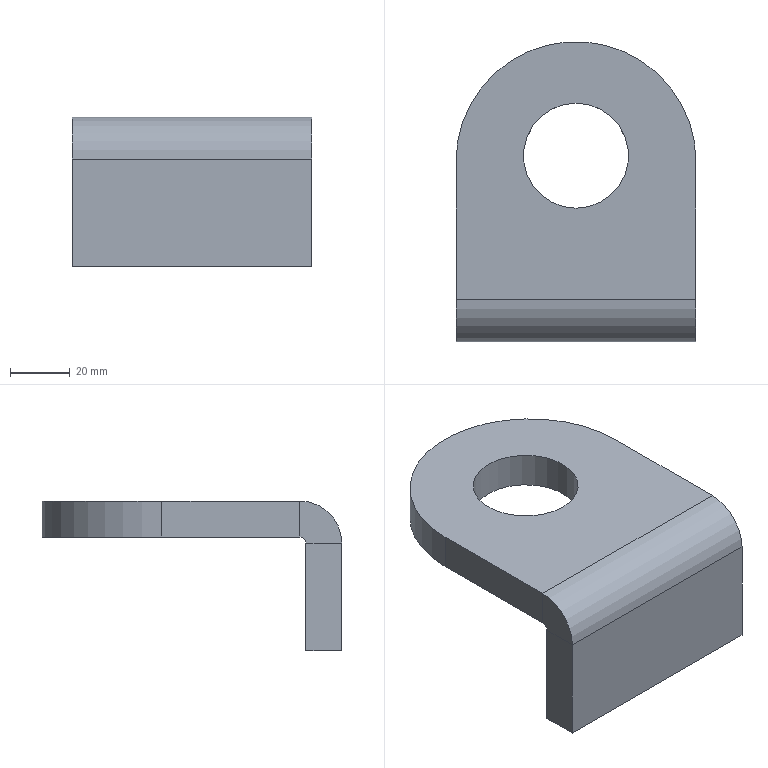Part | STEP file | PN_0019 lifting lug _Default<As Machined> | 1 solid | 15 faces | box 80 x 100 x 50 mm | volume 109398 mm3 | plane 11 | cylinder 4 | commonest cylinder face diameters 4 x1 28 x1 35 x1 80 x1
STEP:
#1=CARTESIAN_POINT('',(0.,0.,0.));
#2=DIRECTION('',(0.,0.,1.));
#3=DIRECTION('',(1.,0.,0.));
#4=AXIS2_PLACEMENT_3D('',#1,#2,#3);
#5=CARTESIAN_POINT('',(-40.,48.,25.));
#6=VERTEX_POINT('',#5);
#7=CARTESIAN_POINT('',(-40.,48.,13.));
#8=VERTEX_POINT('',#7);
#9=CARTESIAN_POINT('',(-40.,48.,25.));
#10=DIRECTION('',(0.,0.,-1.));
#11=VECTOR('',#10,1.);
#12=LINE('',#9,#11);
#13=CARTESIAN_POINT('',(0.,48.,25.));
#14=DIRECTION('',(0.,0.,-1.));
#15=DIRECTION('',(0.,1.,0.));
#16=AXIS2_PLACEMENT_3D('',#13,#14,#15);
#17=CYLINDRICAL_SURFACE('',#16,40.);
#18=CARTESIAN_POINT('',(4.712,0.));
#19=DIRECTION('',(0.,1.));
#20=VECTOR('',#19,1.);
#21=LINE('',#18,#20);
#22=(GEOMETRIC_REPRESENTATION_CONTEXT(2)PARAMETRIC_REPRESENTATION_CONTEXT()REPRESENTATION_CONTEXT('',''));
#23=DEFINITIONAL_REPRESENTATION('',(#21),#22);
#24=PCURVE('',#17,#23);
#25=CARTESIAN_POINT('',(-40.,88.,25.));
#26=DIRECTION('',(-1.,0.,0.));
#27=DIRECTION('',(0.,-1.,0.));
#28=AXIS2_PLACEMENT_3D('',#25,#26,#27);
#29=PLANE('',#28);
#30=CARTESIAN_POINT('',(40.,0.));
#31=DIRECTION('',(0.,-1.));
#32=VECTOR('',#31,1.);
#33=LINE('',#30,#32);
#34=(GEOMETRIC_REPRESENTATION_CONTEXT(2)PARAMETRIC_REPRESENTATION_CONTEXT()REPRESENTATION_CONTEXT('',''));
#35=DEFINITIONAL_REPRESENTATION('',(#33),#34);
#36=PCURVE('',#29,#35);
#37=SURFACE_CURVE('',#12,(#24,#36),.PCURVE_S1.);
#38=EDGE_CURVE('',#6,#8,#37,.T.);
#39=ORIENTED_EDGE('',*,*,#38,.F.);
#40=CARTESIAN_POINT('',(40.,48.,25.));
#41=VERTEX_POINT('',#40);
#42=CARTESIAN_POINT('',(0.,48.,25.));
#43=DIRECTION('',(0.,0.,1.));
#44=DIRECTION('',(0.,-1.,0.));
#45=AXIS2_PLACEMENT_3D('',#42,#43,#44);
#46=CIRCLE('',#45,40.);
#47=CARTESIAN_POINT('',(9.425,0.));
#48=DIRECTION('',(-1.,0.));
#49=VECTOR('',#48,1.);
#50=LINE('',#47,#49);
#51=(GEOMETRIC_REPRESENTATION_CONTEXT(2)PARAMETRIC_REPRESENTATION_CONTEXT()REPRESENTATION_CONTEXT('',''));
#52=DEFINITIONAL_REPRESENTATION('',(#50),#51);
#53=PCURVE('',#17,#52);
#54=CARTESIAN_POINT('',(0.,0.,25.));
#55=DIRECTION('',(0.,0.,1.));
#56=DIRECTION('',(0.,-1.,0.));
#57=AXIS2_PLACEMENT_3D('',#54,#55,#56);
#58=PLANE('',#57);
#59=CARTESIAN_POINT('',(-48.,0.));
#60=DIRECTION('',(1.,0.));
#61=AXIS2_PLACEMENT_2D('',#59,#60);
#62=CIRCLE('',#61,40.);
#63=(GEOMETRIC_REPRESENTATION_CONTEXT(2)PARAMETRIC_REPRESENTATION_CONTEXT()REPRESENTATION_CONTEXT('',''));
#64=DEFINITIONAL_REPRESENTATION('',(#62),#63);
#65=PCURVE('',#58,#64);
#66=SURFACE_CURVE('',#46,(#53,#65),.PCURVE_S1.);
#67=EDGE_CURVE('',#41,#6,#66,.T.);
#68=ORIENTED_EDGE('',*,*,#67,.F.);
#69=CARTESIAN_POINT('',(40.,48.,13.));
#70=VERTEX_POINT('',#69);
#71=CARTESIAN_POINT('',(40.,48.,25.));
#72=DIRECTION('',(0.,0.,1.));
#73=VECTOR('',#72,1.);
#74=LINE('',#71,#73);
#75=CARTESIAN_POINT('',(7.854,0.));
#76=DIRECTION('',(0.,-1.));
#77=VECTOR('',#76,1.);
#78=LINE('',#75,#77);
#79=(GEOMETRIC_REPRESENTATION_CONTEXT(2)PARAMETRIC_REPRESENTATION_CONTEXT()REPRESENTATION_CONTEXT('',''));
#80=DEFINITIONAL_REPRESENTATION('',(#78),#79);
#81=PCURVE('',#17,#80);
#82=CARTESIAN_POINT('',(40.,0.,25.));
#83=DIRECTION('',(1.,0.,0.));
#84=DIRECTION('',(0.,1.,0.));
#85=AXIS2_PLACEMENT_3D('',#82,#83,#84);
#86=PLANE('',#85);
#87=CARTESIAN_POINT('',(48.,0.));
#88=DIRECTION('',(0.,1.));
#89=VECTOR('',#88,1.);
#90=LINE('',#87,#89);
#91=(GEOMETRIC_REPRESENTATION_CONTEXT(2)PARAMETRIC_REPRESENTATION_CONTEXT()REPRESENTATION_CONTEXT('',''));
#92=DEFINITIONAL_REPRESENTATION('',(#90),#91);
#93=PCURVE('',#86,#92);
#94=SURFACE_CURVE('',#74,(#81,#93),.PCURVE_S1.);
#95=EDGE_CURVE('',#70,#41,#94,.T.);
#96=ORIENTED_EDGE('',*,*,#95,.F.);
#97=CARTESIAN_POINT('',(0.,48.,13.));
#98=DIRECTION('',(0.,0.,-1.));
#99=DIRECTION('',(0.,-1.,0.));
#100=AXIS2_PLACEMENT_3D('',#97,#98,#99);
#101=CIRCLE('',#100,40.);
#102=CARTESIAN_POINT('',(3.142,12.));
#103=DIRECTION('',(1.,0.));
#104=VECTOR('',#103,1.);
#105=LINE('',#102,#104);
#106=(GEOMETRIC_REPRESENTATION_CONTEXT(2)PARAMETRIC_REPRESENTATION_CONTEXT()REPRESENTATION_CONTEXT('',''));
#107=DEFINITIONAL_REPRESENTATION('',(#105),#106);
#108=PCURVE('',#17,#107);
#109=CARTESIAN_POINT('',(0.,0.,13.));
#110=DIRECTION('',(0.,0.,1.));
#111=DIRECTION('',(0.,-1.,0.));
#112=AXIS2_PLACEMENT_3D('',#109,#110,#111);
#113=PLANE('',#112);
#114=CARTESIAN_POINT('',(-8.,0.));
#115=CARTESIAN_POINT('',(-8.,-69.282));
#116=CARTESIAN_POINT('',(-68.,-34.641));
#117=CARTESIAN_POINT('',(-128.,0.));
#118=CARTESIAN_POINT('',(-68.,34.641));
#119=CARTESIAN_POINT('',(-8.,69.282));
#120=CARTESIAN_POINT('',(-8.,0.));
#121=(BOUNDED_CURVE()B_SPLINE_CURVE(2,(#114,#115,#116,#117,#118,#119,#120),.UNSPECIFIED.,.T.,.F.)B_SPLINE_CURVE_WITH_KNOTS((1,2,2,2,2,1),(-2.094,0.,2.094,4.189,6.283,8.378),.UNSPECIFIED.)CURVE()GEOMETRIC_REPRESENTATION_ITEM()RATIONAL_B_SPLINE_CURVE((1.,0.5,1.,0.5,1.,0.5,1.))REPRESENTATION_ITEM(''));
#122=(GEOMETRIC_REPRESENTATION_CONTEXT(2)PARAMETRIC_REPRESENTATION_CONTEXT()REPRESENTATION_CONTEXT('',''));
#123=DEFINITIONAL_REPRESENTATION('',(#121),#122);
#124=PCURVE('',#113,#123);
#125=SURFACE_CURVE('',#101,(#108,#124),.PCURVE_S1.);
#126=EDGE_CURVE('',#8,#70,#125,.T.);
#127=ORIENTED_EDGE('',*,*,#126,.F.);
#128=EDGE_LOOP('',(#39,#68,#96,#127));
#129=FACE_BOUND('',#128,.T.);
#130=ADVANCED_FACE('',(#129),#17,.T.);
#131=CARTESIAN_POINT('',(40.,0.,11.));
#132=VERTEX_POINT('',#131);
#133=CARTESIAN_POINT('',(40.,0.,-25.));
#134=VERTEX_POINT('',#133);
#135=CARTESIAN_POINT('',(40.,0.,25.));
#136=DIRECTION('',(0.,0.,-1.));
#137=VECTOR('',#136,1.);
#138=LINE('',#135,#137);
#139=CARTESIAN_POINT('',(40.,-12.,25.));
#140=DIRECTION('',(1.,0.,0.));
#141=DIRECTION('',(0.,0.,-1.));
#142=AXIS2_PLACEMENT_3D('',#139,#140,#141);
#143=PLANE('',#142);
#144=CARTESIAN_POINT('',(0.,12.));
#145=DIRECTION('',(1.,0.));
#146=VECTOR('',#145,1.);
#147=LINE('',#144,#146);
#148=(GEOMETRIC_REPRESENTATION_CONTEXT(2)PARAMETRIC_REPRESENTATION_CONTEXT()REPRESENTATION_CONTEXT('',''));
#149=DEFINITIONAL_REPRESENTATION('',(#147),#148);
#150=PCURVE('',#143,#149);
#151=CARTESIAN_POINT('',(0.,0.,0.));
#152=DIRECTION('',(0.,-1.,0.));
#153=DIRECTION('',(0.,0.,-1.));
#154=AXIS2_PLACEMENT_3D('',#151,#152,#153);
#155=PLANE('',#154);
#156=CARTESIAN_POINT('',(-25.,40.));
#157=DIRECTION('',(1.,0.));
#158=VECTOR('',#157,1.);
#159=LINE('',#156,#158);
#160=(GEOMETRIC_REPRESENTATION_CONTEXT(2)PARAMETRIC_REPRESENTATION_CONTEXT()REPRESENTATION_CONTEXT('',''));
#161=DEFINITIONAL_REPRESENTATION('',(#159),#160);
#162=PCURVE('',#155,#161);
#163=SURFACE_CURVE('',#138,(#150,#162),.PCURVE_S1.);
#164=EDGE_CURVE('',#132,#134,#163,.T.);
#165=ORIENTED_EDGE('',*,*,#164,.F.);
#166=CARTESIAN_POINT('',(40.,-12.,11.));
#167=VERTEX_POINT('',#166);
#168=CARTESIAN_POINT('',(40.,0.,11.));
#169=DIRECTION('',(0.,-1.,0.));
#170=VECTOR('',#169,1.);
#171=LINE('',#168,#170);
#172=CARTESIAN_POINT('',(14.,12.));
#173=DIRECTION('',(0.,-1.));
#174=VECTOR('',#173,1.);
#175=LINE('',#172,#174);
#176=(GEOMETRIC_REPRESENTATION_CONTEXT(2)PARAMETRIC_REPRESENTATION_CONTEXT()REPRESENTATION_CONTEXT('',''));
#177=DEFINITIONAL_REPRESENTATION('',(#175),#176);
#178=PCURVE('',#143,#177);
#179=CARTESIAN_POINT('',(40.,2.,11.));
#180=DIRECTION('',(-1.,0.,0.));
#181=DIRECTION('',(0.,0.,1.));
#182=AXIS2_PLACEMENT_3D('',#179,#180,#181);
#183=PLANE('',#182);
#184=CARTESIAN_POINT('',(0.,-2.));
#185=DIRECTION('',(0.,-1.));
#186=VECTOR('',#185,1.);
#187=LINE('',#184,#186);
#188=(GEOMETRIC_REPRESENTATION_CONTEXT(2)PARAMETRIC_REPRESENTATION_CONTEXT()REPRESENTATION_CONTEXT('',''));
#189=DEFINITIONAL_REPRESENTATION('',(#187),#188);
#190=PCURVE('',#183,#189);
#191=SURFACE_CURVE('',#171,(#178,#190),.PCURVE_S1.);
#192=EDGE_CURVE('',#132,#167,#191,.T.);
#193=ORIENTED_EDGE('',*,*,#192,.T.);
#194=CARTESIAN_POINT('',(40.,-12.,-25.));
#195=VERTEX_POINT('',#194);
#196=CARTESIAN_POINT('',(40.,-12.,25.));
#197=DIRECTION('',(0.,0.,-1.));
#198=VECTOR('',#197,1.);
#199=LINE('',#196,#198);
#200=CARTESIAN_POINT('',(0.,0.));
#201=DIRECTION('',(1.,0.));
#202=VECTOR('',#201,1.);
#203=LINE('',#200,#202);
#204=(GEOMETRIC_REPRESENTATION_CONTEXT(2)PARAMETRIC_REPRESENTATION_CONTEXT()REPRESENTATION_CONTEXT('',''));
#205=DEFINITIONAL_REPRESENTATION('',(#203),#204);
#206=PCURVE('',#143,#205);
#207=CARTESIAN_POINT('',(0.,-12.,0.));
#208=DIRECTION('',(0.,-1.,0.));
#209=DIRECTION('',(0.,0.,-1.));
#210=AXIS2_PLACEMENT_3D('',#207,#208,#209);
#211=PLANE('',#210);
#212=CARTESIAN_POINT('',(-25.,40.));
#213=DIRECTION('',(1.,0.));
#214=VECTOR('',#213,1.);
#215=LINE('',#212,#214);
#216=(GEOMETRIC_REPRESENTATION_CONTEXT(2)PARAMETRIC_REPRESENTATION_CONTEXT()REPRESENTATION_CONTEXT('',''));
#217=DEFINITIONAL_REPRESENTATION('',(#215),#216);
#218=PCURVE('',#211,#217);
#219=SURFACE_CURVE('',#199,(#206,#218),.PCURVE_S1.);
#220=EDGE_CURVE('',#167,#195,#219,.T.);
#221=ORIENTED_EDGE('',*,*,#220,.T.);
#222=CARTESIAN_POINT('',(40.,-12.,-25.));
#223=DIRECTION('',(0.,1.,0.));
#224=VECTOR('',#223,1.);
#225=LINE('',#222,#224);
#226=CARTESIAN_POINT('',(50.,0.));
#227=DIRECTION('',(0.,1.));
#228=VECTOR('',#227,1.);
#229=LINE('',#226,#228);
#230=(GEOMETRIC_REPRESENTATION_CONTEXT(2)PARAMETRIC_REPRESENTATION_CONTEXT()REPRESENTATION_CONTEXT('',''));
#231=DEFINITIONAL_REPRESENTATION('',(#229),#230);
#232=PCURVE('',#143,#231);
#233=CARTESIAN_POINT('',(-40.,-12.,-25.));
#234=DIRECTION('',(0.,0.,-1.));
#235=DIRECTION('',(-1.,0.,0.));
#236=AXIS2_PLACEMENT_3D('',#233,#234,#235);
#237=PLANE('',#236);
#238=CARTESIAN_POINT('',(-80.,0.));
#239=DIRECTION('',(0.,1.));
#240=VECTOR('',#239,1.);
#241=LINE('',#238,#240);
#242=(GEOMETRIC_REPRESENTATION_CONTEXT(2)PARAMETRIC_REPRESENTATION_CONTEXT()REPRESENTATION_CONTEXT('',''));
#243=DEFINITIONAL_REPRESENTATION('',(#241),#242);
#244=PCURVE('',#237,#243);
#245=SURFACE_CURVE('',#225,(#232,#244),.PCURVE_S1.);
#246=EDGE_CURVE('',#195,#134,#245,.T.);
#247=ORIENTED_EDGE('',*,*,#246,.T.);
#248=EDGE_LOOP('',(#165,#193,#221,#247));
#249=FACE_BOUND('',#248,.T.);
#250=ADVANCED_FACE('',(#249),#143,.T.);
#251=ORIENTED_EDGE('',*,*,#220,.F.);
#252=CARTESIAN_POINT('',(-40.,-12.,11.));
#253=VERTEX_POINT('',#252);
#254=CARTESIAN_POINT('',(40.,-12.,11.));
#255=DIRECTION('',(-1.,0.,0.));
#256=VECTOR('',#255,1.);
#257=LINE('',#254,#256);
#258=CARTESIAN_POINT('',(-11.,40.));
#259=DIRECTION('',(0.,-1.));
#260=VECTOR('',#259,1.);
#261=LINE('',#258,#260);
#262=(GEOMETRIC_REPRESENTATION_CONTEXT(2)PARAMETRIC_REPRESENTATION_CONTEXT()REPRESENTATION_CONTEXT('',''));
#263=DEFINITIONAL_REPRESENTATION('',(#261),#262);
#264=PCURVE('',#211,#263);
#265=CARTESIAN_POINT('',(40.,2.,11.));
#266=DIRECTION('',(1.,0.,0.));
#267=DIRECTION('',(0.,0.,1.));
#268=AXIS2_PLACEMENT_3D('',#265,#266,#267);
#269=CYLINDRICAL_SURFACE('',#268,14.);
#270=CARTESIAN_POINT('',(1.571,0.));
#271=DIRECTION('',(0.,-1.));
#272=VECTOR('',#271,1.);
#273=LINE('',#270,#272);
#274=(GEOMETRIC_REPRESENTATION_CONTEXT(2)PARAMETRIC_REPRESENTATION_CONTEXT()REPRESENTATION_CONTEXT('',''));
#275=DEFINITIONAL_REPRESENTATION('',(#273),#274);
#276=PCURVE('',#269,#275);
#277=SURFACE_CURVE('',#257,(#264,#276),.PCURVE_S1.);
#278=EDGE_CURVE('',#167,#253,#277,.T.);
#279=ORIENTED_EDGE('',*,*,#278,.T.);
#280=CARTESIAN_POINT('',(-40.,-12.,-25.));
#281=VERTEX_POINT('',#280);
#282=CARTESIAN_POINT('',(-40.,-12.,25.));
#283=DIRECTION('',(0.,0.,1.));
#284=VECTOR('',#283,1.);
#285=LINE('',#282,#284);
#286=CARTESIAN_POINT('',(-25.,-40.));
#287=DIRECTION('',(-1.,0.));
#288=VECTOR('',#287,1.);
#289=LINE('',#286,#288);
#290=(GEOMETRIC_REPRESENTATION_CONTEXT(2)PARAMETRIC_REPRESENTATION_CONTEXT()REPRESENTATION_CONTEXT('',''));
#291=DEFINITIONAL_REPRESENTATION('',(#289),#290);
#292=PCURVE('',#211,#291);
#293=CARTESIAN_POINT('',(-40.,-12.,25.));
#294=DIRECTION('',(-1.,0.,0.));
#295=DIRECTION('',(0.,0.,1.));
#296=AXIS2_PLACEMENT_3D('',#293,#294,#295);
#297=PLANE('',#296);
#298=CARTESIAN_POINT('',(0.,0.));
#299=DIRECTION('',(1.,0.));
#300=VECTOR('',#299,1.);
#301=LINE('',#298,#300);
#302=(GEOMETRIC_REPRESENTATION_CONTEXT(2)PARAMETRIC_REPRESENTATION_CONTEXT()REPRESENTATION_CONTEXT('',''));
#303=DEFINITIONAL_REPRESENTATION('',(#301),#302);
#304=PCURVE('',#297,#303);
#305=SURFACE_CURVE('',#285,(#292,#304),.PCURVE_S1.);
#306=EDGE_CURVE('',#281,#253,#305,.T.);
#307=ORIENTED_EDGE('',*,*,#306,.F.);
#308=CARTESIAN_POINT('',(-40.,-12.,-25.));
#309=DIRECTION('',(-1.,0.,0.));
#310=VECTOR('',#309,1.);
#311=LINE('',#308,#310);
#312=CARTESIAN_POINT('',(25.,-40.));
#313=DIRECTION('',(0.,-1.));
#314=VECTOR('',#313,1.);
#315=LINE('',#312,#314);
#316=(GEOMETRIC_REPRESENTATION_CONTEXT(2)PARAMETRIC_REPRESENTATION_CONTEXT()REPRESENTATION_CONTEXT('',''));
#317=DEFINITIONAL_REPRESENTATION('',(#315),#316);
#318=PCURVE('',#211,#317);
#319=CARTESIAN_POINT('',(0.,0.));
#320=DIRECTION('',(1.,0.));
#321=VECTOR('',#320,1.);
#322=LINE('',#319,#321);
#323=(GEOMETRIC_REPRESENTATION_CONTEXT(2)PARAMETRIC_REPRESENTATION_CONTEXT()REPRESENTATION_CONTEXT('',''));
#324=DEFINITIONAL_REPRESENTATION('',(#322),#323);
#325=PCURVE('',#237,#324);
#326=SURFACE_CURVE('',#311,(#318,#325),.PCURVE_S1.);
#327=EDGE_CURVE('',#195,#281,#326,.T.);
#328=ORIENTED_EDGE('',*,*,#327,.F.);
#329=EDGE_LOOP('',(#251,#279,#307,#328));
#330=FACE_BOUND('',#329,.T.);
#331=ADVANCED_FACE('',(#330),#211,.T.);
#332=CARTESIAN_POINT('',(-40.,0.,11.));
#333=VERTEX_POINT('',#332);
#334=CARTESIAN_POINT('',(40.,0.,11.));
#335=DIRECTION('',(-1.,0.,0.));
#336=VECTOR('',#335,1.);
#337=LINE('',#334,#336);
#338=CARTESIAN_POINT('',(-11.,40.));
#339=DIRECTION('',(0.,-1.));
#340=VECTOR('',#339,1.);
#341=LINE('',#338,#340);
#342=(GEOMETRIC_REPRESENTATION_CONTEXT(2)PARAMETRIC_REPRESENTATION_CONTEXT()REPRESENTATION_CONTEXT('',''));
#343=DEFINITIONAL_REPRESENTATION('',(#341),#342);
#344=PCURVE('',#155,#343);
#345=CARTESIAN_POINT('',(40.,2.,11.));
#346=DIRECTION('',(1.,0.,0.));
#347=DIRECTION('',(0.,0.,1.));
#348=AXIS2_PLACEMENT_3D('',#345,#346,#347);
#349=CYLINDRICAL_SURFACE('',#348,2.);
#350=CARTESIAN_POINT('',(1.571,0.));
#351=DIRECTION('',(0.,-1.));
#352=VECTOR('',#351,1.);
#353=LINE('',#350,#352);
#354=(GEOMETRIC_REPRESENTATION_CONTEXT(2)PARAMETRIC_REPRESENTATION_CONTEXT()REPRESENTATION_CONTEXT('',''));
#355=DEFINITIONAL_REPRESENTATION('',(#353),#354);
#356=PCURVE('',#349,#355);
#357=SURFACE_CURVE('',#337,(#344,#356),.PCURVE_S1.);
#358=EDGE_CURVE('',#132,#333,#357,.T.);
#359=ORIENTED_EDGE('',*,*,#358,.F.);
#360=ORIENTED_EDGE('',*,*,#164,.T.);
#361=CARTESIAN_POINT('',(-40.,0.,-25.));
#362=VERTEX_POINT('',#361);
#363=CARTESIAN_POINT('',(-40.,0.,-25.));
#364=DIRECTION('',(-1.,0.,0.));
#365=VECTOR('',#364,1.);
#366=LINE('',#363,#365);
#367=CARTESIAN_POINT('',(25.,-40.));
#368=DIRECTION('',(0.,-1.));
#369=VECTOR('',#368,1.);
#370=LINE('',#367,#369);
#371=(GEOMETRIC_REPRESENTATION_CONTEXT(2)PARAMETRIC_REPRESENTATION_CONTEXT()REPRESENTATION_CONTEXT('',''));
#372=DEFINITIONAL_REPRESENTATION('',(#370),#371);
#373=PCURVE('',#155,#372);
#374=CARTESIAN_POINT('',(0.,12.));
#375=DIRECTION('',(1.,0.));
#376=VECTOR('',#375,1.);
#377=LINE('',#374,#376);
#378=(GEOMETRIC_REPRESENTATION_CONTEXT(2)PARAMETRIC_REPRESENTATION_CONTEXT()REPRESENTATION_CONTEXT('',''));
#379=DEFINITIONAL_REPRESENTATION('',(#377),#378);
#380=PCURVE('',#237,#379);
#381=SURFACE_CURVE('',#366,(#373,#380),.PCURVE_S1.);
#382=EDGE_CURVE('',#134,#362,#381,.T.);
#383=ORIENTED_EDGE('',*,*,#382,.T.);
#384=CARTESIAN_POINT('',(-40.,0.,25.));
#385=DIRECTION('',(0.,0.,1.));
#386=VECTOR('',#385,1.);
#387=LINE('',#384,#386);
#388=CARTESIAN_POINT('',(-25.,-40.));
#389=DIRECTION('',(-1.,0.));
#390=VECTOR('',#389,1.);
#391=LINE('',#388,#390);
#392=(GEOMETRIC_REPRESENTATION_CONTEXT(2)PARAMETRIC_REPRESENTATION_CONTEXT()REPRESENTATION_CONTEXT('',''));
#393=DEFINITIONAL_REPRESENTATION('',(#391),#392);
#394=PCURVE('',#155,#393);
#395=CARTESIAN_POINT('',(0.,12.));
#396=DIRECTION('',(1.,0.));
#397=VECTOR('',#396,1.);
#398=LINE('',#395,#397);
#399=(GEOMETRIC_REPRESENTATION_CONTEXT(2)PARAMETRIC_REPRESENTATION_CONTEXT()REPRESENTATION_CONTEXT('',''));
#400=DEFINITIONAL_REPRESENTATION('',(#398),#399);
#401=PCURVE('',#297,#400);
#402=SURFACE_CURVE('',#387,(#394,#401),.PCURVE_S1.);
#403=EDGE_CURVE('',#362,#333,#402,.T.);
#404=ORIENTED_EDGE('',*,*,#403,.T.);
#405=EDGE_LOOP('',(#359,#360,#383,#404));
#406=FACE_BOUND('',#405,.T.);
#407=ADVANCED_FACE('',(#406),#155,.F.);
#408=CARTESIAN_POINT('',(-40.,0.,11.));
#409=DIRECTION('',(0.,-1.,0.));
#410=VECTOR('',#409,1.);
#411=LINE('',#408,#410);
#412=CARTESIAN_POINT('',(-14.,12.));
#413=DIRECTION('',(0.,-1.));
#414=VECTOR('',#413,1.);
#415=LINE('',#412,#414);
#416=(GEOMETRIC_REPRESENTATION_CONTEXT(2)PARAMETRIC_REPRESENTATION_CONTEXT()REPRESENTATION_CONTEXT('',''));
#417=DEFINITIONAL_REPRESENTATION('',(#415),#416);
#418=PCURVE('',#297,#417);
#419=CARTESIAN_POINT('',(-40.,2.,11.));
#420=DIRECTION('',(-1.,0.,0.));
#421=DIRECTION('',(0.,0.,1.));
#422=AXIS2_PLACEMENT_3D('',#419,#420,#421);
#423=PLANE('',#422);
#424=CARTESIAN_POINT('',(0.,-2.));
#425=DIRECTION('',(0.,-1.));
#426=VECTOR('',#425,1.);
#427=LINE('',#424,#426);
#428=(GEOMETRIC_REPRESENTATION_CONTEXT(2)PARAMETRIC_REPRESENTATION_CONTEXT()REPRESENTATION_CONTEXT('',''));
#429=DEFINITIONAL_REPRESENTATION('',(#427),#428);
#430=PCURVE('',#423,#429);
#431=SURFACE_CURVE('',#411,(#418,#430),.PCURVE_S1.);
#432=EDGE_CURVE('',#333,#253,#431,.T.);
#433=ORIENTED_EDGE('',*,*,#432,.F.);
#434=ORIENTED_EDGE('',*,*,#403,.F.);
#435=CARTESIAN_POINT('',(-40.,-12.,-25.));
#436=DIRECTION('',(0.,1.,0.));
#437=VECTOR('',#436,1.);
#438=LINE('',#435,#437);
#439=CARTESIAN_POINT('',(-50.,0.));
#440=DIRECTION('',(0.,1.));
#441=VECTOR('',#440,1.);
#442=LINE('',#439,#441);
#443=(GEOMETRIC_REPRESENTATION_CONTEXT(2)PARAMETRIC_REPRESENTATION_CONTEXT()REPRESENTATION_CONTEXT('',''));
#444=DEFINITIONAL_REPRESENTATION('',(#442),#443);
#445=PCURVE('',#297,#444);
#446=CARTESIAN_POINT('',(0.,0.));
#447=DIRECTION('',(0.,1.));
#448=VECTOR('',#447,1.);
#449=LINE('',#446,#448);
#450=(GEOMETRIC_REPRESENTATION_CONTEXT(2)PARAMETRIC_REPRESENTATION_CONTEXT()REPRESENTATION_CONTEXT('',''));
#451=DEFINITIONAL_REPRESENTATION('',(#449),#450);
#452=PCURVE('',#237,#451);
#453=SURFACE_CURVE('',#438,(#445,#452),.PCURVE_S1.);
#454=EDGE_CURVE('',#281,#362,#453,.T.);
#455=ORIENTED_EDGE('',*,*,#454,.F.);
#456=ORIENTED_EDGE('',*,*,#306,.T.);
#457=EDGE_LOOP('',(#433,#434,#455,#456));
#458=FACE_BOUND('',#457,.T.);
#459=ADVANCED_FACE('',(#458),#297,.T.);
#460=ORIENTED_EDGE('',*,*,#382,.F.);
#461=ORIENTED_EDGE('',*,*,#246,.F.);
#462=ORIENTED_EDGE('',*,*,#327,.T.);
#463=ORIENTED_EDGE('',*,*,#454,.T.);
#464=EDGE_LOOP('',(#460,#461,#462,#463));
#465=FACE_BOUND('',#464,.T.);
#466=ADVANCED_FACE('',(#465),#237,.T.);
#467=CARTESIAN_POINT('',(-40.,2.,13.));
#468=VERTEX_POINT('',#467);
#469=CARTESIAN_POINT('',(-40.,2.,25.));
#470=VERTEX_POINT('',#469);
#471=CARTESIAN_POINT('',(-40.,2.,25.));
#472=DIRECTION('',(0.,0.,1.));
#473=VECTOR('',#472,1.);
#474=LINE('',#471,#473);
#475=CARTESIAN_POINT('',(14.,0.));
#476=DIRECTION('',(1.,0.));
#477=VECTOR('',#476,1.);
#478=LINE('',#475,#477);
#479=(GEOMETRIC_REPRESENTATION_CONTEXT(2)PARAMETRIC_REPRESENTATION_CONTEXT()REPRESENTATION_CONTEXT('',''));
#480=DEFINITIONAL_REPRESENTATION('',(#478),#479);
#481=PCURVE('',#423,#480);
#482=CARTESIAN_POINT('',(86.,0.));
#483=DIRECTION('',(0.,1.));
#484=VECTOR('',#483,1.);
#485=LINE('',#482,#484);
#486=(GEOMETRIC_REPRESENTATION_CONTEXT(2)PARAMETRIC_REPRESENTATION_CONTEXT()REPRESENTATION_CONTEXT('',''));
#487=DEFINITIONAL_REPRESENTATION('',(#485),#486);
#488=PCURVE('',#29,#487);
#489=SURFACE_CURVE('',#474,(#481,#488),.PCURVE_S1.);
#490=EDGE_CURVE('',#468,#470,#489,.T.);
#491=ORIENTED_EDGE('',*,*,#490,.F.);
#492=CARTESIAN_POINT('',(-40.,2.,11.));
#493=DIRECTION('',(-1.,0.,0.));
#494=DIRECTION('',(0.,0.,-1.));
#495=AXIS2_PLACEMENT_3D('',#492,#493,#494);
#496=CIRCLE('',#495,2.);
#497=CARTESIAN_POINT('',(0.,0.));
#498=DIRECTION('',(-1.,0.));
#499=AXIS2_PLACEMENT_2D('',#497,#498);
#500=CIRCLE('',#499,2.);
#501=(GEOMETRIC_REPRESENTATION_CONTEXT(2)PARAMETRIC_REPRESENTATION_CONTEXT()REPRESENTATION_CONTEXT('',''));
#502=DEFINITIONAL_REPRESENTATION('',(#500),#501);
#503=PCURVE('',#423,#502);
#504=CARTESIAN_POINT('',(3.142,-80.));
#505=DIRECTION('',(-1.,0.));
#506=VECTOR('',#505,1.);
#507=LINE('',#504,#506);
#508=(GEOMETRIC_REPRESENTATION_CONTEXT(2)PARAMETRIC_REPRESENTATION_CONTEXT()REPRESENTATION_CONTEXT('',''));
#509=DEFINITIONAL_REPRESENTATION('',(#507),#508);
#510=PCURVE('',#349,#509);
#511=SURFACE_CURVE('',#496,(#503,#510),.PCURVE_S1.);
#512=EDGE_CURVE('',#333,#468,#511,.T.);
#513=ORIENTED_EDGE('',*,*,#512,.F.);
#514=ORIENTED_EDGE('',*,*,#432,.T.);
#515=CARTESIAN_POINT('',(-40.,2.,11.));
#516=DIRECTION('',(-1.,0.,0.));
#517=DIRECTION('',(0.,0.,-1.));
#518=AXIS2_PLACEMENT_3D('',#515,#516,#517);
#519=CIRCLE('',#518,14.);
#520=CARTESIAN_POINT('',(0.,0.));
#521=DIRECTION('',(-1.,0.));
#522=AXIS2_PLACEMENT_2D('',#520,#521);
#523=CIRCLE('',#522,14.);
#524=(GEOMETRIC_REPRESENTATION_CONTEXT(2)PARAMETRIC_REPRESENTATION_CONTEXT()REPRESENTATION_CONTEXT('',''));
#525=DEFINITIONAL_REPRESENTATION('',(#523),#524);
#526=PCURVE('',#423,#525);
#527=CARTESIAN_POINT('',(3.142,-80.));
#528=DIRECTION('',(-1.,0.));
#529=VECTOR('',#528,1.);
#530=LINE('',#527,#529);
#531=(GEOMETRIC_REPRESENTATION_CONTEXT(2)PARAMETRIC_REPRESENTATION_CONTEXT()REPRESENTATION_CONTEXT('',''));
#532=DEFINITIONAL_REPRESENTATION('',(#530),#531);
#533=PCURVE('',#269,#532);
#534=SURFACE_CURVE('',#519,(#526,#533),.PCURVE_S1.);
#535=EDGE_CURVE('',#253,#470,#534,.T.);
#536=ORIENTED_EDGE('',*,*,#535,.T.);
#537=EDGE_LOOP('',(#491,#513,#514,#536));
#538=FACE_BOUND('',#537,.T.);
#539=ADVANCED_FACE('',(#538),#423,.T.);
#540=CARTESIAN_POINT('',(40.,2.,13.));
#541=VERTEX_POINT('',#540);
#542=CARTESIAN_POINT('',(40.,2.,11.));
#543=DIRECTION('',(1.,0.,0.));
#544=DIRECTION('',(0.,0.,-1.));
#545=AXIS2_PLACEMENT_3D('',#542,#543,#544);
#546=CIRCLE('',#545,2.);
#547=CARTESIAN_POINT('',(-2.,0.));
#548=CARTESIAN_POINT('',(-2.,3.464));
#549=CARTESIAN_POINT('',(1.,1.732));
#550=CARTESIAN_POINT('',(4.,0.));
#551=CARTESIAN_POINT('',(1.,-1.732));
#552=CARTESIAN_POINT('',(-2.,-3.464));
#553=CARTESIAN_POINT('',(-2.,0.));
#554=(BOUNDED_CURVE()B_SPLINE_CURVE(2,(#547,#548,#549,#550,#551,#552,#553),.UNSPECIFIED.,.T.,.F.)B_SPLINE_CURVE_WITH_KNOTS((1,2,2,2,2,1),(-2.094,0.,2.094,4.189,6.283,8.378),.UNSPECIFIED.)CURVE()GEOMETRIC_REPRESENTATION_ITEM()RATIONAL_B_SPLINE_CURVE((1.,0.5,1.,0.5,1.,0.5,1.))REPRESENTATION_ITEM(''));
#555=(GEOMETRIC_REPRESENTATION_CONTEXT(2)PARAMETRIC_REPRESENTATION_CONTEXT()REPRESENTATION_CONTEXT('',''));
#556=DEFINITIONAL_REPRESENTATION('',(#554),#555);
#557=PCURVE('',#183,#556);
#558=CARTESIAN_POINT('',(-3.142,0.));
#559=DIRECTION('',(1.,0.));
#560=VECTOR('',#559,1.);
#561=LINE('',#558,#560);
#562=(GEOMETRIC_REPRESENTATION_CONTEXT(2)PARAMETRIC_REPRESENTATION_CONTEXT()REPRESENTATION_CONTEXT('',''));
#563=DEFINITIONAL_REPRESENTATION('',(#561),#562);
#564=PCURVE('',#349,#563);
#565=SURFACE_CURVE('',#546,(#557,#564),.PCURVE_S1.);
#566=EDGE_CURVE('',#541,#132,#565,.T.);
#567=ORIENTED_EDGE('',*,*,#566,.F.);
#568=CARTESIAN_POINT('',(40.,2.,25.));
#569=VERTEX_POINT('',#568);
#570=CARTESIAN_POINT('',(40.,2.,13.));
#571=DIRECTION('',(0.,0.,1.));
#572=VECTOR('',#571,1.);
#573=LINE('',#570,#572);
#574=CARTESIAN_POINT('',(2.,0.));
#575=DIRECTION('',(1.,0.));
#576=VECTOR('',#575,1.);
#577=LINE('',#574,#576);
#578=(GEOMETRIC_REPRESENTATION_CONTEXT(2)PARAMETRIC_REPRESENTATION_CONTEXT()REPRESENTATION_CONTEXT('',''));
#579=DEFINITIONAL_REPRESENTATION('',(#577),#578);
#580=PCURVE('',#183,#579);
#581=CARTESIAN_POINT('',(2.,-12.));
#582=DIRECTION('',(0.,1.));
#583=VECTOR('',#582,1.);
#584=LINE('',#581,#583);
#585=(GEOMETRIC_REPRESENTATION_CONTEXT(2)PARAMETRIC_REPRESENTATION_CONTEXT()REPRESENTATION_CONTEXT('',''));
#586=DEFINITIONAL_REPRESENTATION('',(#584),#585);
#587=PCURVE('',#86,#586);
#588=SURFACE_CURVE('',#573,(#580,#587),.PCURVE_S1.);
#589=EDGE_CURVE('',#541,#569,#588,.T.);
#590=ORIENTED_EDGE('',*,*,#589,.T.);
#591=CARTESIAN_POINT('',(40.,2.,11.));
#592=DIRECTION('',(1.,0.,0.));
#593=DIRECTION('',(0.,0.,-1.));
#594=AXIS2_PLACEMENT_3D('',#591,#592,#593);
#595=CIRCLE('',#594,14.);
#596=CARTESIAN_POINT('',(-14.,0.));
#597=CARTESIAN_POINT('',(-14.,24.249));
#598=CARTESIAN_POINT('',(7.,12.124));
#599=CARTESIAN_POINT('',(28.,0.));
#600=CARTESIAN_POINT('',(7.,-12.124));
#601=CARTESIAN_POINT('',(-14.,-24.249));
#602=CARTESIAN_POINT('',(-14.,0.));
#603=(BOUNDED_CURVE()B_SPLINE_CURVE(2,(#596,#597,#598,#599,#600,#601,#602),.UNSPECIFIED.,.T.,.F.)B_SPLINE_CURVE_WITH_KNOTS((1,2,2,2,2,1),(-2.094,0.,2.094,4.189,6.283,8.378),.UNSPECIFIED.)CURVE()GEOMETRIC_REPRESENTATION_ITEM()RATIONAL_B_SPLINE_CURVE((1.,0.5,1.,0.5,1.,0.5,1.))REPRESENTATION_ITEM(''));
#604=(GEOMETRIC_REPRESENTATION_CONTEXT(2)PARAMETRIC_REPRESENTATION_CONTEXT()REPRESENTATION_CONTEXT('',''));
#605=DEFINITIONAL_REPRESENTATION('',(#603),#604);
#606=PCURVE('',#183,#605);
#607=CARTESIAN_POINT('',(-3.142,0.));
#608=DIRECTION('',(1.,0.));
#609=VECTOR('',#608,1.);
#610=LINE('',#607,#609);
#611=(GEOMETRIC_REPRESENTATION_CONTEXT(2)PARAMETRIC_REPRESENTATION_CONTEXT()REPRESENTATION_CONTEXT('',''));
#612=DEFINITIONAL_REPRESENTATION('',(#610),#611);
#613=PCURVE('',#269,#612);
#614=SURFACE_CURVE('',#595,(#606,#613),.PCURVE_S1.);
#615=EDGE_CURVE('',#569,#167,#614,.T.);
#616=ORIENTED_EDGE('',*,*,#615,.T.);
#617=ORIENTED_EDGE('',*,*,#192,.F.);
#618=EDGE_LOOP('',(#567,#590,#616,#617));
#619=FACE_BOUND('',#618,.T.);
#620=ADVANCED_FACE('',(#619),#183,.F.);
#621=ORIENTED_EDGE('',*,*,#278,.F.);
#622=ORIENTED_EDGE('',*,*,#615,.F.);
#623=CARTESIAN_POINT('',(0.,2.,25.));
#624=DIRECTION('',(1.,0.,0.));
#625=VECTOR('',#624,1.);
#626=LINE('',#623,#625);
#627=CARTESIAN_POINT('',(0.,-40.));
#628=DIRECTION('',(0.,1.));
#629=VECTOR('',#628,1.);
#630=LINE('',#627,#629);
#631=(GEOMETRIC_REPRESENTATION_CONTEXT(2)PARAMETRIC_REPRESENTATION_CONTEXT()REPRESENTATION_CONTEXT('',''));
#632=DEFINITIONAL_REPRESENTATION('',(#630),#631);
#633=PCURVE('',#269,#632);
#634=CARTESIAN_POINT('',(-2.,0.));
#635=DIRECTION('',(0.,1.));
#636=VECTOR('',#635,1.);
#637=LINE('',#634,#636);
#638=(GEOMETRIC_REPRESENTATION_CONTEXT(2)PARAMETRIC_REPRESENTATION_CONTEXT()REPRESENTATION_CONTEXT('',''));
#639=DEFINITIONAL_REPRESENTATION('',(#637),#638);
#640=PCURVE('',#58,#639);
#641=SURFACE_CURVE('',#626,(#633,#640),.PCURVE_S1.);
#642=EDGE_CURVE('',#470,#569,#641,.T.);
#643=ORIENTED_EDGE('',*,*,#642,.F.);
#644=ORIENTED_EDGE('',*,*,#535,.F.);
#645=EDGE_LOOP('',(#621,#622,#643,#644));
#646=FACE_BOUND('',#645,.T.);
#647=ADVANCED_FACE('',(#646),#269,.T.);
#648=ORIENTED_EDGE('',*,*,#566,.F.);
#649=CARTESIAN_POINT('',(-40.,2.,13.));
#650=DIRECTION('',(1.,0.,0.));
#651=VECTOR('',#650,1.);
#652=LINE('',#649,#651);
#653=CARTESIAN_POINT('',(0.,-80.));
#654=DIRECTION('',(0.,1.));
#655=VECTOR('',#654,1.);
#656=LINE('',#653,#655);
#657=(GEOMETRIC_REPRESENTATION_CONTEXT(2)PARAMETRIC_REPRESENTATION_CONTEXT()REPRESENTATION_CONTEXT('',''));
#658=DEFINITIONAL_REPRESENTATION('',(#656),#657);
#659=PCURVE('',#349,#658);
#660=CARTESIAN_POINT('',(-2.,-40.));
#661=DIRECTION('',(0.,1.));
#662=VECTOR('',#661,1.);
#663=LINE('',#660,#662);
#664=(GEOMETRIC_REPRESENTATION_CONTEXT(2)PARAMETRIC_REPRESENTATION_CONTEXT()REPRESENTATION_CONTEXT('',''));
#665=DEFINITIONAL_REPRESENTATION('',(#663),#664);
#666=PCURVE('',#113,#665);
#667=SURFACE_CURVE('',#652,(#659,#666),.PCURVE_S1.);
#668=EDGE_CURVE('',#468,#541,#667,.T.);
#669=ORIENTED_EDGE('',*,*,#668,.F.);
#670=ORIENTED_EDGE('',*,*,#512,.F.);
#671=ORIENTED_EDGE('',*,*,#358,.F.);
#672=EDGE_LOOP('',(#648,#669,#670,#671));
#673=FACE_BOUND('',#672,.F.);
#674=ADVANCED_FACE('',(#673),#349,.F.);
#675=CARTESIAN_POINT('',(40.,0.,13.));
#676=DIRECTION('',(0.,-1.,0.));
#677=VECTOR('',#676,1.);
#678=LINE('',#675,#677);
#679=CARTESIAN_POINT('',(0.,-12.));
#680=DIRECTION('',(-1.,0.));
#681=VECTOR('',#680,1.);
#682=LINE('',#679,#681);
#683=(GEOMETRIC_REPRESENTATION_CONTEXT(2)PARAMETRIC_REPRESENTATION_CONTEXT()REPRESENTATION_CONTEXT('',''));
#684=DEFINITIONAL_REPRESENTATION('',(#682),#683);
#685=PCURVE('',#86,#684);
#686=CARTESIAN_POINT('',(0.,40.));
#687=DIRECTION('',(1.,0.));
#688=VECTOR('',#687,1.);
#689=LINE('',#686,#688);
#690=(GEOMETRIC_REPRESENTATION_CONTEXT(2)PARAMETRIC_REPRESENTATION_CONTEXT()REPRESENTATION_CONTEXT('',''));
#691=DEFINITIONAL_REPRESENTATION('',(#689),#690);
#692=PCURVE('',#113,#691);
#693=SURFACE_CURVE('',#678,(#685,#692),.PCURVE_S1.);
#694=EDGE_CURVE('',#70,#541,#693,.T.);
#695=ORIENTED_EDGE('',*,*,#694,.F.);
#696=ORIENTED_EDGE('',*,*,#95,.T.);
#697=CARTESIAN_POINT('',(40.,0.,25.));
#698=DIRECTION('',(0.,-1.,0.));
#699=VECTOR('',#698,1.);
#700=LINE('',#697,#699);
#701=CARTESIAN_POINT('',(0.,0.));
#702=DIRECTION('',(-1.,0.));
#703=VECTOR('',#702,1.);
#704=LINE('',#701,#703);
#705=(GEOMETRIC_REPRESENTATION_CONTEXT(2)PARAMETRIC_REPRESENTATION_CONTEXT()REPRESENTATION_CONTEXT('',''));
#706=DEFINITIONAL_REPRESENTATION('',(#704),#705);
#707=PCURVE('',#86,#706);
#708=CARTESIAN_POINT('',(0.,40.));
#709=DIRECTION('',(1.,0.));
#710=VECTOR('',#709,1.);
#711=LINE('',#708,#710);
#712=(GEOMETRIC_REPRESENTATION_CONTEXT(2)PARAMETRIC_REPRESENTATION_CONTEXT()REPRESENTATION_CONTEXT('',''));
#713=DEFINITIONAL_REPRESENTATION('',(#711),#712);
#714=PCURVE('',#58,#713);
#715=SURFACE_CURVE('',#700,(#707,#714),.PCURVE_S1.);
#716=EDGE_CURVE('',#41,#569,#715,.T.);
#717=ORIENTED_EDGE('',*,*,#716,.T.);
#718=ORIENTED_EDGE('',*,*,#589,.F.);
#719=EDGE_LOOP('',(#695,#696,#717,#718));
#720=FACE_BOUND('',#719,.T.);
#721=ADVANCED_FACE('',(#720),#86,.T.);
#722=CARTESIAN_POINT('',(-40.,88.,25.));
#723=DIRECTION('',(0.,1.,0.));
#724=VECTOR('',#723,1.);
#725=LINE('',#722,#724);
#726=CARTESIAN_POINT('',(0.,0.));
#727=DIRECTION('',(-1.,0.));
#728=VECTOR('',#727,1.);
#729=LINE('',#726,#728);
#730=(GEOMETRIC_REPRESENTATION_CONTEXT(2)PARAMETRIC_REPRESENTATION_CONTEXT()REPRESENTATION_CONTEXT('',''));
#731=DEFINITIONAL_REPRESENTATION('',(#729),#730);
#732=PCURVE('',#29,#731);
#733=CARTESIAN_POINT('',(-88.,-40.));
#734=DIRECTION('',(-1.,0.));
#735=VECTOR('',#734,1.);
#736=LINE('',#733,#735);
#737=(GEOMETRIC_REPRESENTATION_CONTEXT(2)PARAMETRIC_REPRESENTATION_CONTEXT()REPRESENTATION_CONTEXT('',''));
#738=DEFINITIONAL_REPRESENTATION('',(#736),#737);
#739=PCURVE('',#58,#738);
#740=SURFACE_CURVE('',#725,(#732,#739),.PCURVE_S1.);
#741=EDGE_CURVE('',#470,#6,#740,.T.);
#742=ORIENTED_EDGE('',*,*,#741,.T.);
#743=ORIENTED_EDGE('',*,*,#38,.T.);
#744=CARTESIAN_POINT('',(-40.,0.,13.));
#745=DIRECTION('',(0.,1.,0.));
#746=VECTOR('',#745,1.);
#747=LINE('',#744,#746);
#748=CARTESIAN_POINT('',(88.,-12.));
#749=DIRECTION('',(-1.,0.));
#750=VECTOR('',#749,1.);
#751=LINE('',#748,#750);
#752=(GEOMETRIC_REPRESENTATION_CONTEXT(2)PARAMETRIC_REPRESENTATION_CONTEXT()REPRESENTATION_CONTEXT('',''));
#753=DEFINITIONAL_REPRESENTATION('',(#751),#752);
#754=PCURVE('',#29,#753);
#755=CARTESIAN_POINT('',(0.,-40.));
#756=DIRECTION('',(-1.,0.));
#757=VECTOR('',#756,1.);
#758=LINE('',#755,#757);
#759=(GEOMETRIC_REPRESENTATION_CONTEXT(2)PARAMETRIC_REPRESENTATION_CONTEXT()REPRESENTATION_CONTEXT('',''));
#760=DEFINITIONAL_REPRESENTATION('',(#758),#759);
#761=PCURVE('',#113,#760);
#762=SURFACE_CURVE('',#747,(#754,#761),.PCURVE_S1.);
#763=EDGE_CURVE('',#468,#8,#762,.T.);
#764=ORIENTED_EDGE('',*,*,#763,.F.);
#765=ORIENTED_EDGE('',*,*,#490,.T.);
#766=EDGE_LOOP('',(#742,#743,#764,#765));
#767=FACE_BOUND('',#766,.T.);
#768=ADVANCED_FACE('',(#767),#29,.T.);
#769=CARTESIAN_POINT('',(0.,32.5,25.));
#770=VERTEX_POINT('',#769);
#771=CARTESIAN_POINT('',(0.,67.5,25.));
#772=VERTEX_POINT('',#771);
#773=CARTESIAN_POINT('',(0.,50.,25.));
#774=DIRECTION('',(0.,0.,1.));
#775=DIRECTION('',(0.,-1.,0.));
#776=AXIS2_PLACEMENT_3D('',#773,#774,#775);
#777=CIRCLE('',#776,17.5);
#778=CARTESIAN_POINT('',(-50.,0.));
#779=DIRECTION('',(1.,0.));
#780=AXIS2_PLACEMENT_2D('',#778,#779);
#781=CIRCLE('',#780,17.5);
#782=(GEOMETRIC_REPRESENTATION_CONTEXT(2)PARAMETRIC_REPRESENTATION_CONTEXT()REPRESENTATION_CONTEXT('',''));
#783=DEFINITIONAL_REPRESENTATION('',(#781),#782);
#784=PCURVE('',#58,#783);
#785=CARTESIAN_POINT('',(0.,50.,13.));
#786=DIRECTION('',(0.,0.,-1.));
#787=DIRECTION('',(0.,1.,0.));
#788=AXIS2_PLACEMENT_3D('',#785,#786,#787);
#789=CYLINDRICAL_SURFACE('',#788,17.5);
#790=CARTESIAN_POINT('',(3.142,-12.));
#791=DIRECTION('',(-1.,0.));
#792=VECTOR('',#791,1.);
#793=LINE('',#790,#792);
#794=(GEOMETRIC_REPRESENTATION_CONTEXT(2)PARAMETRIC_REPRESENTATION_CONTEXT()REPRESENTATION_CONTEXT('',''));
#795=DEFINITIONAL_REPRESENTATION('',(#793),#794);
#796=PCURVE('',#789,#795);
#797=SURFACE_CURVE('',#777,(#784,#796),.PCURVE_S1.);
#798=EDGE_CURVE('',#770,#772,#797,.T.);
#799=ORIENTED_EDGE('',*,*,#798,.F.);
#800=CARTESIAN_POINT('',(0.,50.,25.));
#801=DIRECTION('',(0.,0.,1.));
#802=DIRECTION('',(0.,-1.,0.));
#803=AXIS2_PLACEMENT_3D('',#800,#801,#802);
#804=CIRCLE('',#803,17.5);
#805=CARTESIAN_POINT('',(-50.,0.));
#806=DIRECTION('',(1.,0.));
#807=AXIS2_PLACEMENT_2D('',#805,#806);
#808=CIRCLE('',#807,17.5);
#809=(GEOMETRIC_REPRESENTATION_CONTEXT(2)PARAMETRIC_REPRESENTATION_CONTEXT()REPRESENTATION_CONTEXT('',''));
#810=DEFINITIONAL_REPRESENTATION('',(#808),#809);
#811=PCURVE('',#58,#810);
#812=CARTESIAN_POINT('',(9.425,-12.));
#813=DIRECTION('',(-1.,0.));
#814=VECTOR('',#813,1.);
#815=LINE('',#812,#814);
#816=(GEOMETRIC_REPRESENTATION_CONTEXT(2)PARAMETRIC_REPRESENTATION_CONTEXT()REPRESENTATION_CONTEXT('',''));
#817=DEFINITIONAL_REPRESENTATION('',(#815),#816);
#818=PCURVE('',#789,#817);
#819=SURFACE_CURVE('',#804,(#811,#818),.PCURVE_S1.);
#820=EDGE_CURVE('',#772,#770,#819,.T.);
#821=ORIENTED_EDGE('',*,*,#820,.F.);
#822=EDGE_LOOP('',(#799,#821));
#823=FACE_BOUND('',#822,.T.);
#824=ORIENTED_EDGE('',*,*,#716,.F.);
#825=ORIENTED_EDGE('',*,*,#67,.T.);
#826=ORIENTED_EDGE('',*,*,#741,.F.);
#827=ORIENTED_EDGE('',*,*,#642,.T.);
#828=EDGE_LOOP('',(#824,#825,#826,#827));
#829=FACE_BOUND('',#828,.T.);
#830=ADVANCED_FACE('',(#823,#829),#58,.T.);
#831=CARTESIAN_POINT('',(0.,67.5,13.));
#832=VERTEX_POINT('',#831);
#833=CARTESIAN_POINT('',(0.,50.,13.));
#834=DIRECTION('',(0.,0.,-1.));
#835=DIRECTION('',(0.,1.,0.));
#836=AXIS2_PLACEMENT_3D('',#833,#834,#835);
#837=CIRCLE('',#836,17.5);
#838=CARTESIAN_POINT('',(-67.5,0.));
#839=CARTESIAN_POINT('',(-67.5,30.311));
#840=CARTESIAN_POINT('',(-41.25,15.155));
#841=CARTESIAN_POINT('',(-15.,0.));
#842=CARTESIAN_POINT('',(-41.25,-15.155));
#843=CARTESIAN_POINT('',(-67.5,-30.311));
#844=CARTESIAN_POINT('',(-67.5,0.));
#845=(BOUNDED_CURVE()B_SPLINE_CURVE(2,(#838,#839,#840,#841,#842,#843,#844),.UNSPECIFIED.,.T.,.F.)B_SPLINE_CURVE_WITH_KNOTS((1,2,2,2,2,1),(-2.094,0.,2.094,4.189,6.283,8.378),.UNSPECIFIED.)CURVE()GEOMETRIC_REPRESENTATION_ITEM()RATIONAL_B_SPLINE_CURVE((1.,0.5,1.,0.5,1.,0.5,1.))REPRESENTATION_ITEM(''));
#846=(GEOMETRIC_REPRESENTATION_CONTEXT(2)PARAMETRIC_REPRESENTATION_CONTEXT()REPRESENTATION_CONTEXT('',''));
#847=DEFINITIONAL_REPRESENTATION('',(#845),#846);
#848=PCURVE('',#113,#847);
#849=CARTESIAN_POINT('',(0.,0.));
#850=DIRECTION('',(1.,0.));
#851=VECTOR('',#850,1.);
#852=LINE('',#849,#851);
#853=(GEOMETRIC_REPRESENTATION_CONTEXT(2)PARAMETRIC_REPRESENTATION_CONTEXT()REPRESENTATION_CONTEXT('',''));
#854=DEFINITIONAL_REPRESENTATION('',(#852),#853);
#855=PCURVE('',#789,#854);
#856=SURFACE_CURVE('',#837,(#848,#855),.PCURVE_S1.);
#857=EDGE_CURVE('',#832,#832,#856,.T.);
#858=ORIENTED_EDGE('',*,*,#857,.F.);
#859=EDGE_LOOP('',(#858));
#860=FACE_BOUND('',#859,.T.);
#861=ORIENTED_EDGE('',*,*,#763,.T.);
#862=ORIENTED_EDGE('',*,*,#126,.T.);
#863=ORIENTED_EDGE('',*,*,#694,.T.);
#864=ORIENTED_EDGE('',*,*,#668,.F.);
#865=EDGE_LOOP('',(#861,#862,#863,#864));
#866=FACE_BOUND('',#865,.T.);
#867=ADVANCED_FACE('',(#860,#866),#113,.F.);
#868=ORIENTED_EDGE('',*,*,#857,.F.);
#869=CARTESIAN_POINT('',(0.,67.5,25.));
#870=CARTESIAN_POINT('',(0.,67.5,13.));
#871=B_SPLINE_CURVE_WITH_KNOTS('',1,(#869,#870),.UNSPECIFIED.,.F.,.F.,(2,2),(-12.,0.),.PIECEWISE_BEZIER_KNOTS.);
#872=CARTESIAN_POINT('',(0.,0.));
#873=DIRECTION('',(0.,1.));
#874=VECTOR('',#873,1.);
#875=LINE('',#872,#874);
#876=(GEOMETRIC_REPRESENTATION_CONTEXT(2)PARAMETRIC_REPRESENTATION_CONTEXT()REPRESENTATION_CONTEXT('',''));
#877=DEFINITIONAL_REPRESENTATION('',(#875),#876);
#878=PCURVE('',#789,#877);
#879=CARTESIAN_POINT('',(6.283,0.));
#880=DIRECTION('',(0.,1.));
#881=VECTOR('',#880,1.);
#882=LINE('',#879,#881);
#883=(GEOMETRIC_REPRESENTATION_CONTEXT(2)PARAMETRIC_REPRESENTATION_CONTEXT()REPRESENTATION_CONTEXT('',''));
#884=DEFINITIONAL_REPRESENTATION('',(#882),#883);
#885=PCURVE('',#789,#884);
#886=SEAM_CURVE('',#871,(#878,#885),.PCURVE_S1.);
#887=EDGE_CURVE('',#772,#832,#886,.T.);
#888=ORIENTED_EDGE('',*,*,#887,.F.);
#889=ORIENTED_EDGE('',*,*,#798,.F.);
#890=ORIENTED_EDGE('',*,*,#820,.F.);
#891=ORIENTED_EDGE('',*,*,#887,.T.);
#892=EDGE_LOOP('',(#868,#888,#889,#890,#891));
#893=FACE_BOUND('',#892,.F.);
#894=ADVANCED_FACE('',(#893),#789,.F.);
#895=CLOSED_SHELL('',(#130,#250,#331,#407,#459,#466,#539,#620,#647,#674,#721,#768,#830,#867,#894));
#896=MANIFOLD_SOLID_BREP('',#895);
#897=(LENGTH_UNIT()NAMED_UNIT(*)SI_UNIT(.MILLI.,.METRE.));
#898=UNCERTAINTY_MEASURE_WITH_UNIT(LENGTH_MEASURE(0.000001),#897,'','');
#899=(NAMED_UNIT(*)PLANE_ANGLE_UNIT()SI_UNIT($,.RADIAN.));
#900=(NAMED_UNIT(*)SI_UNIT($,.STERADIAN.)SOLID_ANGLE_UNIT());
#901=(GEOMETRIC_REPRESENTATION_CONTEXT(3)GLOBAL_UNCERTAINTY_ASSIGNED_CONTEXT((#898))GLOBAL_UNIT_ASSIGNED_CONTEXT((#897,#899,#900))REPRESENTATION_CONTEXT('',''));
#902=ADVANCED_BREP_SHAPE_REPRESENTATION('',(#4,#896),#901);